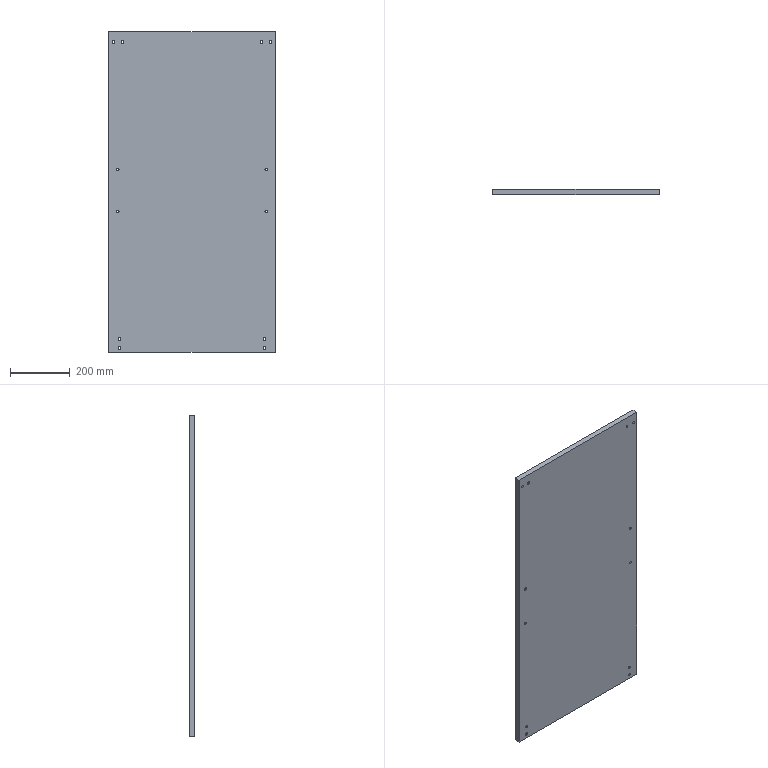Part | STEP file | DECK509 | 1 solid | 26 faces | box 554 x 18 x 1070 mm | volume 10652247 mm3 | cylinder 16 | plane 10 | commonest cylinder face diameters 8.5 x12 18 x4